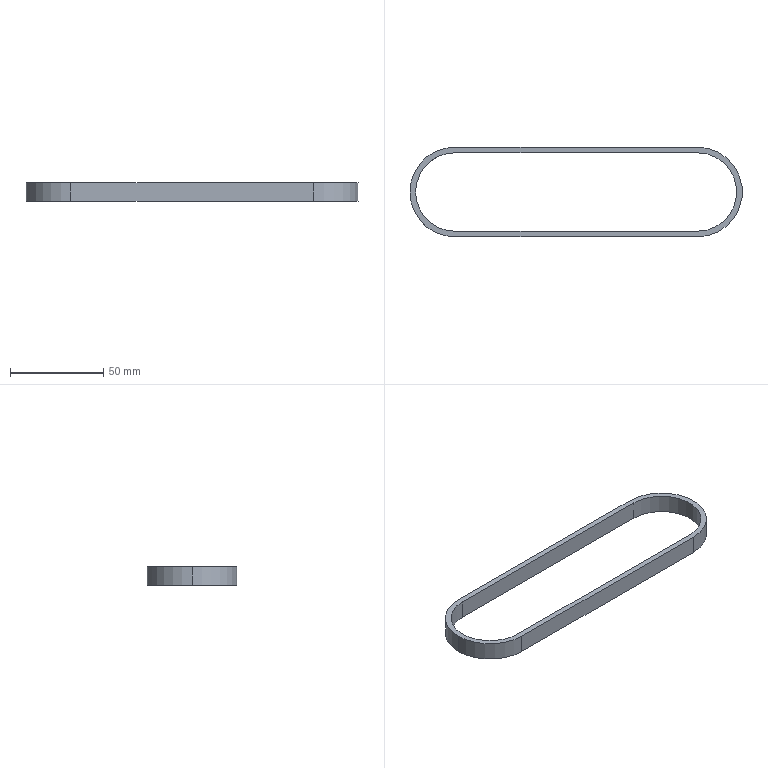Part | SolidWorks | features Extrusion 1, Shell 1 | 1 solid | 12 faces | box 178 x 48 x 10 mm | volume 12041 mm3 | cylinder 6 | plane 6 | commonest cylinder face diameters 42 x3 48 x3
STEP:
#1=CARTESIAN_POINT('',(-130.,21.,10.));
#2=VERTEX_POINT('',#1);
#3=CARTESIAN_POINT('',(-151.,0.,10.));
#4=VERTEX_POINT('',#3);
#5=CARTESIAN_POINT('',(-130.,0.,10.));
#6=DIRECTION('',(0.,0.,1.));
#7=DIRECTION('',(1.,0.,0.));
#8=AXIS2_PLACEMENT_3D('',#5,#6,#7);
#9=CIRCLE('',#8,21.);
#10=EDGE_CURVE('',#2,#4,#9,.T.);
#11=ORIENTED_EDGE('',*,*,#10,.T.);
#12=CARTESIAN_POINT('',(-151.,0.,0.));
#13=VERTEX_POINT('',#12);
#14=CARTESIAN_POINT('',(-151.,0.,10.));
#15=DIRECTION('',(0.,0.,-1.));
#16=VECTOR('',#15,1000.);
#17=LINE('',#14,#16);
#18=EDGE_CURVE('',#4,#13,#17,.T.);
#19=ORIENTED_EDGE('',*,*,#18,.T.);
#20=CARTESIAN_POINT('',(-130.,21.,0.));
#21=VERTEX_POINT('',#20);
#22=CARTESIAN_POINT('',(-130.,0.,0.));
#23=DIRECTION('',(0.,0.,1.));
#24=DIRECTION('',(1.,0.,0.));
#25=AXIS2_PLACEMENT_3D('',#22,#23,#24);
#26=CIRCLE('',#25,21.);
#27=EDGE_CURVE('',#21,#13,#26,.T.);
#28=ORIENTED_EDGE('',*,*,#27,.F.);
#29=CARTESIAN_POINT('',(-130.,21.,10.));
#30=DIRECTION('',(0.,0.,-1.));
#31=VECTOR('',#30,1000.);
#32=LINE('',#29,#31);
#33=EDGE_CURVE('',#2,#21,#32,.T.);
#34=ORIENTED_EDGE('',*,*,#33,.F.);
#35=EDGE_LOOP('',(#11,#19,#28,#34));
#36=FACE_OUTER_BOUND('',#35,.T.);
#37=CARTESIAN_POINT('',(-130.,0.,10.));
#38=DIRECTION('',(0.,0.,-1.));
#39=DIRECTION('',(-1.,0.,0.));
#40=AXIS2_PLACEMENT_3D('',#37,#38,#39);
#41=CYLINDRICAL_SURFACE('',#40,21.);
#42=ADVANCED_FACE('',(#36),#41,.F.);
#43=CARTESIAN_POINT('',(-154.,0.,10.));
#44=VERTEX_POINT('',#43);
#45=CARTESIAN_POINT('',(-130.,-24.,10.));
#46=VERTEX_POINT('',#45);
#47=CARTESIAN_POINT('',(-130.,0.,10.));
#48=DIRECTION('',(0.,0.,1.));
#49=DIRECTION('',(1.,0.,0.));
#50=AXIS2_PLACEMENT_3D('',#47,#48,#49);
#51=CIRCLE('',#50,24.);
#52=EDGE_CURVE('',#44,#46,#51,.T.);
#53=ORIENTED_EDGE('',*,*,#52,.F.);
#54=CARTESIAN_POINT('',(-154.,0.,0.));
#55=VERTEX_POINT('',#54);
#56=CARTESIAN_POINT('',(-154.,0.,10.));
#57=DIRECTION('',(0.,0.,-1.));
#58=VECTOR('',#57,1000.);
#59=LINE('',#56,#58);
#60=EDGE_CURVE('',#44,#55,#59,.T.);
#61=ORIENTED_EDGE('',*,*,#60,.T.);
#62=CARTESIAN_POINT('',(-130.,-24.,0.));
#63=VERTEX_POINT('',#62);
#64=CARTESIAN_POINT('',(-130.,0.,0.));
#65=DIRECTION('',(0.,0.,1.));
#66=DIRECTION('',(1.,0.,0.));
#67=AXIS2_PLACEMENT_3D('',#64,#65,#66);
#68=CIRCLE('',#67,24.);
#69=EDGE_CURVE('',#55,#63,#68,.T.);
#70=ORIENTED_EDGE('',*,*,#69,.T.);
#71=CARTESIAN_POINT('',(-130.,-24.,10.));
#72=DIRECTION('',(0.,0.,-1.));
#73=VECTOR('',#72,1000.);
#74=LINE('',#71,#73);
#75=EDGE_CURVE('',#46,#63,#74,.T.);
#76=ORIENTED_EDGE('',*,*,#75,.F.);
#77=EDGE_LOOP('',(#53,#61,#70,#76));
#78=FACE_OUTER_BOUND('',#77,.T.);
#79=CARTESIAN_POINT('',(-130.,0.,10.));
#80=DIRECTION('',(0.,0.,-1.));
#81=DIRECTION('',(-1.,0.,0.));
#82=AXIS2_PLACEMENT_3D('',#79,#80,#81);
#83=CYLINDRICAL_SURFACE('',#82,24.);
#84=ADVANCED_FACE('',(#78),#83,.T.);
#85=CARTESIAN_POINT('',(0.,-24.,0.));
#86=VERTEX_POINT('',#85);
#87=CARTESIAN_POINT('',(0.,24.,0.));
#88=VERTEX_POINT('',#87);
#89=CARTESIAN_POINT('',(0.,0.,0.));
#90=DIRECTION('',(0.,0.,1.));
#91=DIRECTION('',(1.,0.,0.));
#92=AXIS2_PLACEMENT_3D('',#89,#90,#91);
#93=CIRCLE('',#92,24.);
#94=EDGE_CURVE('',#86,#88,#93,.T.);
#95=ORIENTED_EDGE('',*,*,#94,.T.);
#96=CARTESIAN_POINT('',(0.,24.,10.));
#97=VERTEX_POINT('',#96);
#98=CARTESIAN_POINT('',(0.,24.,10.));
#99=DIRECTION('',(0.,0.,-1.));
#100=VECTOR('',#99,1000.);
#101=LINE('',#98,#100);
#102=EDGE_CURVE('',#97,#88,#101,.T.);
#103=ORIENTED_EDGE('',*,*,#102,.F.);
#104=CARTESIAN_POINT('',(0.,-24.,10.));
#105=VERTEX_POINT('',#104);
#106=CARTESIAN_POINT('',(0.,0.,10.));
#107=DIRECTION('',(0.,0.,1.));
#108=DIRECTION('',(1.,0.,0.));
#109=AXIS2_PLACEMENT_3D('',#106,#107,#108);
#110=CIRCLE('',#109,24.);
#111=EDGE_CURVE('',#105,#97,#110,.T.);
#112=ORIENTED_EDGE('',*,*,#111,.F.);
#113=CARTESIAN_POINT('',(0.,-24.,10.));
#114=DIRECTION('',(0.,0.,-1.));
#115=VECTOR('',#114,1000.);
#116=LINE('',#113,#115);
#117=EDGE_CURVE('',#105,#86,#116,.T.);
#118=ORIENTED_EDGE('',*,*,#117,.T.);
#119=EDGE_LOOP('',(#95,#103,#112,#118));
#120=FACE_OUTER_BOUND('',#119,.T.);
#121=CARTESIAN_POINT('',(0.,0.,10.));
#122=DIRECTION('',(0.,0.,-1.));
#123=DIRECTION('',(-1.,0.,0.));
#124=AXIS2_PLACEMENT_3D('',#121,#122,#123);
#125=CYLINDRICAL_SURFACE('',#124,24.);
#126=ADVANCED_FACE('',(#120),#125,.T.);
#127=CARTESIAN_POINT('',(-130.,24.,0.));
#128=VERTEX_POINT('',#127);
#129=CARTESIAN_POINT('',(0.,24.,0.));
#130=DIRECTION('',(-1.,0.,0.));
#131=VECTOR('',#130,1000.);
#132=LINE('',#129,#131);
#133=EDGE_CURVE('',#88,#128,#132,.T.);
#134=ORIENTED_EDGE('',*,*,#133,.T.);
#135=CARTESIAN_POINT('',(-130.,24.,10.));
#136=VERTEX_POINT('',#135);
#137=CARTESIAN_POINT('',(-130.,24.,10.));
#138=DIRECTION('',(0.,0.,-1.));
#139=VECTOR('',#138,1000.);
#140=LINE('',#137,#139);
#141=EDGE_CURVE('',#136,#128,#140,.T.);
#142=ORIENTED_EDGE('',*,*,#141,.F.);
#143=CARTESIAN_POINT('',(0.,24.,10.));
#144=DIRECTION('',(-1.,0.,0.));
#145=VECTOR('',#144,1000.);
#146=LINE('',#143,#145);
#147=EDGE_CURVE('',#97,#136,#146,.T.);
#148=ORIENTED_EDGE('',*,*,#147,.F.);
#149=ORIENTED_EDGE('',*,*,#102,.T.);
#150=EDGE_LOOP('',(#134,#142,#148,#149));
#151=FACE_OUTER_BOUND('',#150,.T.);
#152=CARTESIAN_POINT('',(0.,24.,10.));
#153=DIRECTION('',(0.,-1.,0.));
#154=DIRECTION('',(0.,0.,-1.));
#155=AXIS2_PLACEMENT_3D('',#152,#153,#154);
#156=PLANE('',#155);
#157=ADVANCED_FACE('',(#151),#156,.F.);
#158=ORIENTED_EDGE('',*,*,#60,.F.);
#159=CARTESIAN_POINT('',(-130.,0.,10.));
#160=DIRECTION('',(0.,0.,1.));
#161=DIRECTION('',(1.,0.,0.));
#162=AXIS2_PLACEMENT_3D('',#159,#160,#161);
#163=CIRCLE('',#162,24.);
#164=EDGE_CURVE('',#136,#44,#163,.T.);
#165=ORIENTED_EDGE('',*,*,#164,.F.);
#166=ORIENTED_EDGE('',*,*,#141,.T.);
#167=CARTESIAN_POINT('',(-130.,0.,0.));
#168=DIRECTION('',(0.,0.,1.));
#169=DIRECTION('',(1.,0.,0.));
#170=AXIS2_PLACEMENT_3D('',#167,#168,#169);
#171=CIRCLE('',#170,24.);
#172=EDGE_CURVE('',#128,#55,#171,.T.);
#173=ORIENTED_EDGE('',*,*,#172,.T.);
#174=EDGE_LOOP('',(#158,#165,#166,#173));
#175=FACE_OUTER_BOUND('',#174,.T.);
#176=CARTESIAN_POINT('',(-130.,0.,10.));
#177=DIRECTION('',(0.,0.,-1.));
#178=DIRECTION('',(-1.,0.,0.));
#179=AXIS2_PLACEMENT_3D('',#176,#177,#178);
#180=CYLINDRICAL_SURFACE('',#179,24.);
#181=ADVANCED_FACE('',(#175),#180,.T.);
#182=CARTESIAN_POINT('',(0.,-24.,0.));
#183=DIRECTION('',(1.,0.,0.));
#184=VECTOR('',#183,1000.);
#185=LINE('',#182,#184);
#186=EDGE_CURVE('',#63,#86,#185,.T.);
#187=ORIENTED_EDGE('',*,*,#186,.T.);
#188=ORIENTED_EDGE('',*,*,#117,.F.);
#189=CARTESIAN_POINT('',(0.,-24.,10.));
#190=DIRECTION('',(1.,0.,0.));
#191=VECTOR('',#190,1000.);
#192=LINE('',#189,#191);
#193=EDGE_CURVE('',#46,#105,#192,.T.);
#194=ORIENTED_EDGE('',*,*,#193,.F.);
#195=ORIENTED_EDGE('',*,*,#75,.T.);
#196=EDGE_LOOP('',(#187,#188,#194,#195));
#197=FACE_OUTER_BOUND('',#196,.T.);
#198=CARTESIAN_POINT('',(0.,-24.,10.));
#199=DIRECTION('',(0.,1.,0.));
#200=DIRECTION('',(0.,0.,1.));
#201=AXIS2_PLACEMENT_3D('',#198,#199,#200);
#202=PLANE('',#201);
#203=ADVANCED_FACE('',(#197),#202,.F.);
#204=CARTESIAN_POINT('',(0.,-21.,10.));
#205=VERTEX_POINT('',#204);
#206=CARTESIAN_POINT('',(0.,21.,10.));
#207=VERTEX_POINT('',#206);
#208=CARTESIAN_POINT('',(0.,0.,10.));
#209=DIRECTION('',(0.,0.,1.));
#210=DIRECTION('',(1.,0.,0.));
#211=AXIS2_PLACEMENT_3D('',#208,#209,#210);
#212=CIRCLE('',#211,21.);
#213=EDGE_CURVE('',#205,#207,#212,.T.);
#214=ORIENTED_EDGE('',*,*,#213,.F.);
#215=CARTESIAN_POINT('',(-130.,-21.,10.));
#216=VERTEX_POINT('',#215);
#217=CARTESIAN_POINT('',(0.,-21.,10.));
#218=DIRECTION('',(1.,0.,0.));
#219=VECTOR('',#218,1000.);
#220=LINE('',#217,#219);
#221=EDGE_CURVE('',#216,#205,#220,.T.);
#222=ORIENTED_EDGE('',*,*,#221,.F.);
#223=CARTESIAN_POINT('',(-130.,0.,10.));
#224=DIRECTION('',(0.,0.,1.));
#225=DIRECTION('',(1.,0.,0.));
#226=AXIS2_PLACEMENT_3D('',#223,#224,#225);
#227=CIRCLE('',#226,21.);
#228=EDGE_CURVE('',#4,#216,#227,.T.);
#229=ORIENTED_EDGE('',*,*,#228,.F.);
#230=ORIENTED_EDGE('',*,*,#10,.F.);
#231=CARTESIAN_POINT('',(0.,21.,10.));
#232=DIRECTION('',(-1.,0.,0.));
#233=VECTOR('',#232,1000.);
#234=LINE('',#231,#233);
#235=EDGE_CURVE('',#207,#2,#234,.T.);
#236=ORIENTED_EDGE('',*,*,#235,.F.);
#237=EDGE_LOOP('',(#214,#222,#229,#230,#236));
#238=FACE_BOUND('',#237,.T.);
#239=ORIENTED_EDGE('',*,*,#111,.T.);
#240=ORIENTED_EDGE('',*,*,#147,.T.);
#241=ORIENTED_EDGE('',*,*,#164,.T.);
#242=ORIENTED_EDGE('',*,*,#52,.T.);
#243=ORIENTED_EDGE('',*,*,#193,.T.);
#244=EDGE_LOOP('',(#239,#240,#241,#242,#243));
#245=FACE_OUTER_BOUND('',#244,.T.);
#246=CARTESIAN_POINT('',(0.,0.,10.));
#247=DIRECTION('',(0.,0.,1.));
#248=DIRECTION('',(1.,0.,0.));
#249=AXIS2_PLACEMENT_3D('',#246,#247,#248);
#250=PLANE('',#249);
#251=ADVANCED_FACE('',(#238,#245),#250,.T.);
#252=CARTESIAN_POINT('',(-130.,-21.,0.));
#253=VERTEX_POINT('',#252);
#254=CARTESIAN_POINT('',(0.,-21.,0.));
#255=VERTEX_POINT('',#254);
#256=CARTESIAN_POINT('',(0.,-21.,0.));
#257=DIRECTION('',(1.,0.,0.));
#258=VECTOR('',#257,1000.);
#259=LINE('',#256,#258);
#260=EDGE_CURVE('',#253,#255,#259,.T.);
#261=ORIENTED_EDGE('',*,*,#260,.T.);
#262=CARTESIAN_POINT('',(0.,21.,0.));
#263=VERTEX_POINT('',#262);
#264=CARTESIAN_POINT('',(0.,0.,0.));
#265=DIRECTION('',(0.,0.,1.));
#266=DIRECTION('',(1.,0.,0.));
#267=AXIS2_PLACEMENT_3D('',#264,#265,#266);
#268=CIRCLE('',#267,21.);
#269=EDGE_CURVE('',#255,#263,#268,.T.);
#270=ORIENTED_EDGE('',*,*,#269,.T.);
#271=CARTESIAN_POINT('',(0.,21.,0.));
#272=DIRECTION('',(-1.,0.,0.));
#273=VECTOR('',#272,1000.);
#274=LINE('',#271,#273);
#275=EDGE_CURVE('',#263,#21,#274,.T.);
#276=ORIENTED_EDGE('',*,*,#275,.T.);
#277=ORIENTED_EDGE('',*,*,#27,.T.);
#278=CARTESIAN_POINT('',(-130.,0.,0.));
#279=DIRECTION('',(0.,0.,1.));
#280=DIRECTION('',(1.,0.,0.));
#281=AXIS2_PLACEMENT_3D('',#278,#279,#280);
#282=CIRCLE('',#281,21.);
#283=EDGE_CURVE('',#13,#253,#282,.T.);
#284=ORIENTED_EDGE('',*,*,#283,.T.);
#285=EDGE_LOOP('',(#261,#270,#276,#277,#284));
#286=FACE_BOUND('',#285,.T.);
#287=ORIENTED_EDGE('',*,*,#94,.F.);
#288=ORIENTED_EDGE('',*,*,#186,.F.);
#289=ORIENTED_EDGE('',*,*,#69,.F.);
#290=ORIENTED_EDGE('',*,*,#172,.F.);
#291=ORIENTED_EDGE('',*,*,#133,.F.);
#292=EDGE_LOOP('',(#287,#288,#289,#290,#291));
#293=FACE_OUTER_BOUND('',#292,.T.);
#294=CARTESIAN_POINT('',(0.,0.,0.));
#295=DIRECTION('',(0.,0.,1.));
#296=DIRECTION('',(1.,0.,0.));
#297=AXIS2_PLACEMENT_3D('',#294,#295,#296);
#298=PLANE('',#297);
#299=ADVANCED_FACE('',(#286,#293),#298,.F.);
#300=ORIENTED_EDGE('',*,*,#269,.F.);
#301=CARTESIAN_POINT('',(0.,-21.,10.));
#302=DIRECTION('',(0.,0.,-1.));
#303=VECTOR('',#302,1000.);
#304=LINE('',#301,#303);
#305=EDGE_CURVE('',#205,#255,#304,.T.);
#306=ORIENTED_EDGE('',*,*,#305,.F.);
#307=ORIENTED_EDGE('',*,*,#213,.T.);
#308=CARTESIAN_POINT('',(0.,21.,10.));
#309=DIRECTION('',(0.,0.,-1.));
#310=VECTOR('',#309,1000.);
#311=LINE('',#308,#310);
#312=EDGE_CURVE('',#207,#263,#311,.T.);
#313=ORIENTED_EDGE('',*,*,#312,.T.);
#314=EDGE_LOOP('',(#300,#306,#307,#313));
#315=FACE_OUTER_BOUND('',#314,.T.);
#316=CARTESIAN_POINT('',(0.,0.,10.));
#317=DIRECTION('',(0.,0.,-1.));
#318=DIRECTION('',(-1.,0.,0.));
#319=AXIS2_PLACEMENT_3D('',#316,#317,#318);
#320=CYLINDRICAL_SURFACE('',#319,21.);
#321=ADVANCED_FACE('',(#315),#320,.F.);
#322=ORIENTED_EDGE('',*,*,#275,.F.);
#323=ORIENTED_EDGE('',*,*,#312,.F.);
#324=ORIENTED_EDGE('',*,*,#235,.T.);
#325=ORIENTED_EDGE('',*,*,#33,.T.);
#326=EDGE_LOOP('',(#322,#323,#324,#325));
#327=FACE_OUTER_BOUND('',#326,.T.);
#328=CARTESIAN_POINT('',(0.,21.,10.));
#329=DIRECTION('',(0.,-1.,0.));
#330=DIRECTION('',(0.,0.,-1.));
#331=AXIS2_PLACEMENT_3D('',#328,#329,#330);
#332=PLANE('',#331);
#333=ADVANCED_FACE('',(#327),#332,.T.);
#334=ORIENTED_EDGE('',*,*,#18,.F.);
#335=ORIENTED_EDGE('',*,*,#228,.T.);
#336=CARTESIAN_POINT('',(-130.,-21.,10.));
#337=DIRECTION('',(0.,0.,-1.));
#338=VECTOR('',#337,1000.);
#339=LINE('',#336,#338);
#340=EDGE_CURVE('',#216,#253,#339,.T.);
#341=ORIENTED_EDGE('',*,*,#340,.T.);
#342=ORIENTED_EDGE('',*,*,#283,.F.);
#343=EDGE_LOOP('',(#334,#335,#341,#342));
#344=FACE_OUTER_BOUND('',#343,.T.);
#345=CARTESIAN_POINT('',(-130.,0.,10.));
#346=DIRECTION('',(0.,0.,-1.));
#347=DIRECTION('',(-1.,0.,0.));
#348=AXIS2_PLACEMENT_3D('',#345,#346,#347);
#349=CYLINDRICAL_SURFACE('',#348,21.);
#350=ADVANCED_FACE('',(#344),#349,.F.);
#351=ORIENTED_EDGE('',*,*,#260,.F.);
#352=ORIENTED_EDGE('',*,*,#340,.F.);
#353=ORIENTED_EDGE('',*,*,#221,.T.);
#354=ORIENTED_EDGE('',*,*,#305,.T.);
#355=EDGE_LOOP('',(#351,#352,#353,#354));
#356=FACE_OUTER_BOUND('',#355,.T.);
#357=CARTESIAN_POINT('',(0.,-21.,10.));
#358=DIRECTION('',(0.,1.,0.));
#359=DIRECTION('',(0.,0.,1.));
#360=AXIS2_PLACEMENT_3D('',#357,#358,#359);
#361=PLANE('',#360);
#362=ADVANCED_FACE('',(#356),#361,.T.);
#363=CLOSED_SHELL('',(#42,#84,#126,#157,#181,#203,#251,#299,#321,#333,#350,#362));
#364=MANIFOLD_SOLID_BREP('',#363);
#365=CARTESIAN_POINT('',(0.,0.,0.));
#366=DIRECTION('',(0.,0.,1.));
#367=DIRECTION('',(1.,0.,0.));
#368=AXIS2_PLACEMENT_3D('',#365,#366,#367);
#369=(LENGTH_UNIT()NAMED_UNIT(*)SI_UNIT(.MILLI.,.METRE.));
#370=UNCERTAINTY_MEASURE_WITH_UNIT(LENGTH_MEASURE(0.00001),#369,'','');
#371=(NAMED_UNIT(*)PLANE_ANGLE_UNIT()SI_UNIT($,.RADIAN.));
#372=(NAMED_UNIT(*)SI_UNIT($,.STERADIAN.)SOLID_ANGLE_UNIT());
#373=(GEOMETRIC_REPRESENTATION_CONTEXT(3)GLOBAL_UNCERTAINTY_ASSIGNED_CONTEXT((#370))GLOBAL_UNIT_ASSIGNED_CONTEXT((#369,#371,#372))REPRESENTATION_CONTEXT('',''));
#374=ADVANCED_BREP_SHAPE_REPRESENTATION('',(#364,#368),#373);